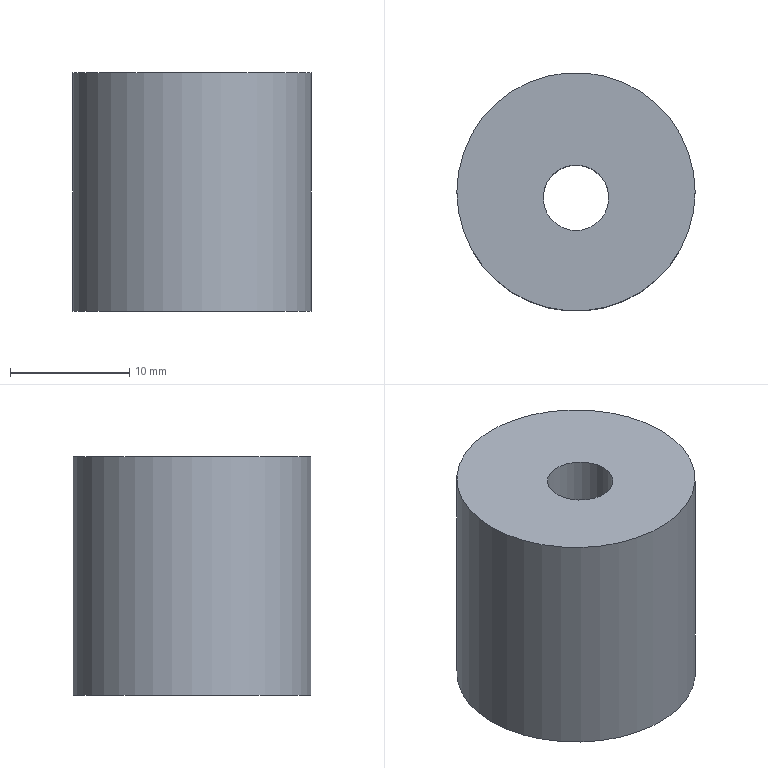Part | STEP file | solid 188 | 1 solid | 6 faces | box 20 x 20 x 20 mm | volume 5479 mm3 | plane 3 | cylinder 3 | commonest cylinder face diameters 5.5 x1 10 x1 20 x1